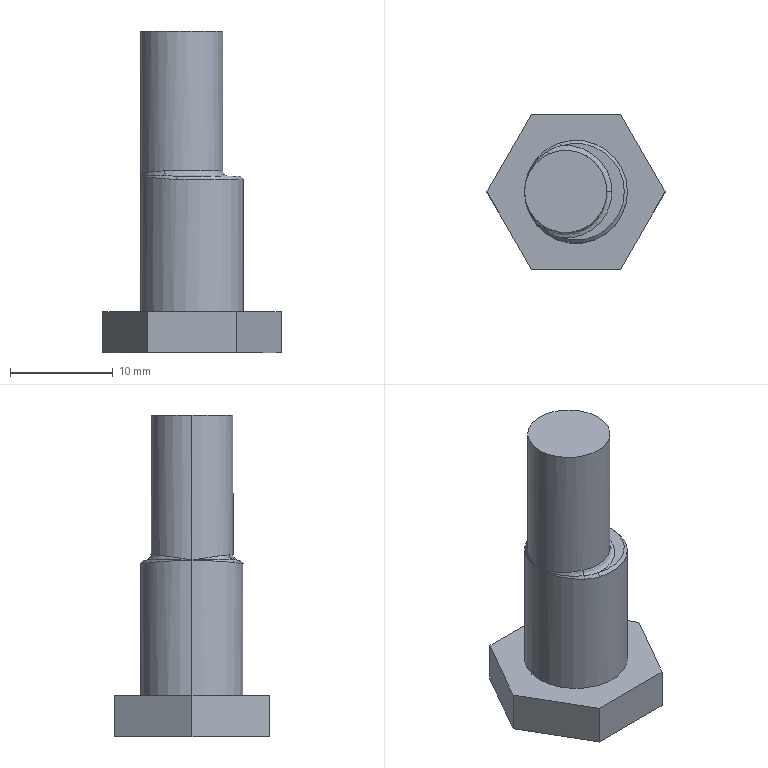Part | SolidWorks | features BaseBody 1 | 1 solid | 23 faces | box 17.321 x 15 x 31.3 mm | volume 2525 mm3 | plane 10 | spline 8 | cylinder 4 | cone 1 | commonest cylinder face diameters 8 x2 10 x2